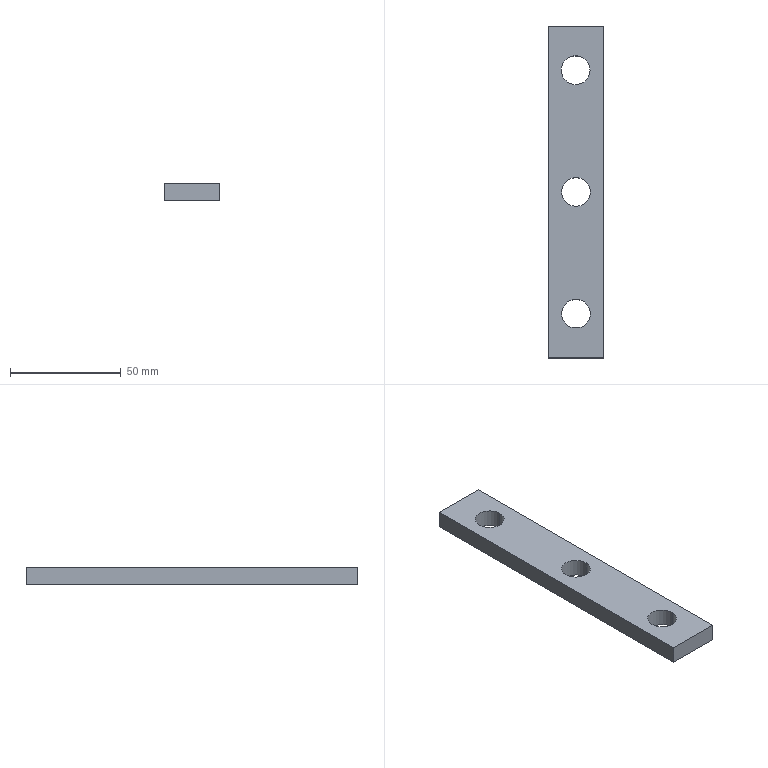Part | SolidWorks | features Extrusion 1 | 1 solid | 12 faces | box 25 x 150 x 8 mm | volume 26814 mm3 | cylinder 6 | plane 6 | commonest cylinder face diameters 13 x6
STEP:
#1=CARTESIAN_POINT('',(-6.5,-55.,8.));
#2=VERTEX_POINT('',#1);
#3=CARTESIAN_POINT('',(6.5,-55.,8.));
#4=VERTEX_POINT('',#3);
#5=CARTESIAN_POINT('',(0.,-55.,8.));
#6=DIRECTION('',(0.,0.,1.));
#7=DIRECTION('',(1.,0.,0.));
#8=AXIS2_PLACEMENT_3D('',#5,#6,#7);
#9=CIRCLE('',#8,6.5);
#10=EDGE_CURVE('',#2,#4,#9,.T.);
#11=ORIENTED_EDGE('',*,*,#10,.T.);
#12=CARTESIAN_POINT('',(6.5,-55.,0.));
#13=VERTEX_POINT('',#12);
#14=CARTESIAN_POINT('',(6.5,-55.,8.));
#15=DIRECTION('',(0.,0.,-1.));
#16=VECTOR('',#15,1000.);
#17=LINE('',#14,#16);
#18=EDGE_CURVE('',#4,#13,#17,.T.);
#19=ORIENTED_EDGE('',*,*,#18,.T.);
#20=CARTESIAN_POINT('',(-6.5,-55.,0.));
#21=VERTEX_POINT('',#20);
#22=CARTESIAN_POINT('',(0.,-55.,0.));
#23=DIRECTION('',(0.,0.,1.));
#24=DIRECTION('',(1.,0.,0.));
#25=AXIS2_PLACEMENT_3D('',#22,#23,#24);
#26=CIRCLE('',#25,6.5);
#27=EDGE_CURVE('',#21,#13,#26,.T.);
#28=ORIENTED_EDGE('',*,*,#27,.F.);
#29=CARTESIAN_POINT('',(-6.5,-55.,8.));
#30=DIRECTION('',(0.,0.,-1.));
#31=VECTOR('',#30,1000.);
#32=LINE('',#29,#31);
#33=EDGE_CURVE('',#2,#21,#32,.T.);
#34=ORIENTED_EDGE('',*,*,#33,.F.);
#35=EDGE_LOOP('',(#11,#19,#28,#34));
#36=FACE_OUTER_BOUND('',#35,.T.);
#37=CARTESIAN_POINT('',(0.,-55.,8.));
#38=DIRECTION('',(0.,0.,-1.));
#39=DIRECTION('',(-1.,0.,0.));
#40=AXIS2_PLACEMENT_3D('',#37,#38,#39);
#41=CYLINDRICAL_SURFACE('',#40,6.5);
#42=ADVANCED_FACE('',(#36),#41,.F.);
#43=CARTESIAN_POINT('',(-6.5,0.,8.));
#44=VERTEX_POINT('',#43);
#45=CARTESIAN_POINT('',(6.5,0.,8.));
#46=VERTEX_POINT('',#45);
#47=CARTESIAN_POINT('',(0.,0.,8.));
#48=DIRECTION('',(0.,0.,1.));
#49=DIRECTION('',(1.,0.,0.));
#50=AXIS2_PLACEMENT_3D('',#47,#48,#49);
#51=CIRCLE('',#50,6.5);
#52=EDGE_CURVE('',#44,#46,#51,.T.);
#53=ORIENTED_EDGE('',*,*,#52,.T.);
#54=CARTESIAN_POINT('',(6.5,0.,0.));
#55=VERTEX_POINT('',#54);
#56=CARTESIAN_POINT('',(6.5,0.,8.));
#57=DIRECTION('',(0.,0.,-1.));
#58=VECTOR('',#57,1000.);
#59=LINE('',#56,#58);
#60=EDGE_CURVE('',#46,#55,#59,.T.);
#61=ORIENTED_EDGE('',*,*,#60,.T.);
#62=CARTESIAN_POINT('',(-6.5,0.,0.));
#63=VERTEX_POINT('',#62);
#64=CARTESIAN_POINT('',(0.,0.,0.));
#65=DIRECTION('',(0.,0.,1.));
#66=DIRECTION('',(1.,0.,0.));
#67=AXIS2_PLACEMENT_3D('',#64,#65,#66);
#68=CIRCLE('',#67,6.5);
#69=EDGE_CURVE('',#63,#55,#68,.T.);
#70=ORIENTED_EDGE('',*,*,#69,.F.);
#71=CARTESIAN_POINT('',(-6.5,0.,8.));
#72=DIRECTION('',(0.,0.,-1.));
#73=VECTOR('',#72,1000.);
#74=LINE('',#71,#73);
#75=EDGE_CURVE('',#44,#63,#74,.T.);
#76=ORIENTED_EDGE('',*,*,#75,.F.);
#77=EDGE_LOOP('',(#53,#61,#70,#76));
#78=FACE_OUTER_BOUND('',#77,.T.);
#79=CARTESIAN_POINT('',(0.,0.,8.));
#80=DIRECTION('',(0.,0.,-1.));
#81=DIRECTION('',(-1.,0.,0.));
#82=AXIS2_PLACEMENT_3D('',#79,#80,#81);
#83=CYLINDRICAL_SURFACE('',#82,6.5);
#84=ADVANCED_FACE('',(#78),#83,.F.);
#85=CARTESIAN_POINT('',(-6.654,55.,8.));
#86=VERTEX_POINT('',#85);
#87=CARTESIAN_POINT('',(6.346,55.,8.));
#88=VERTEX_POINT('',#87);
#89=CARTESIAN_POINT('',(-0.1539,55.,8.));
#90=DIRECTION('',(0.,0.,1.));
#91=DIRECTION('',(1.,0.,0.));
#92=AXIS2_PLACEMENT_3D('',#89,#90,#91);
#93=CIRCLE('',#92,6.5);
#94=EDGE_CURVE('',#86,#88,#93,.T.);
#95=ORIENTED_EDGE('',*,*,#94,.T.);
#96=CARTESIAN_POINT('',(6.346,55.,0.));
#97=VERTEX_POINT('',#96);
#98=CARTESIAN_POINT('',(6.346,55.,8.));
#99=DIRECTION('',(0.,0.,-1.));
#100=VECTOR('',#99,1000.);
#101=LINE('',#98,#100);
#102=EDGE_CURVE('',#88,#97,#101,.T.);
#103=ORIENTED_EDGE('',*,*,#102,.T.);
#104=CARTESIAN_POINT('',(-6.654,55.,0.));
#105=VERTEX_POINT('',#104);
#106=CARTESIAN_POINT('',(-0.1539,55.,0.));
#107=DIRECTION('',(0.,0.,1.));
#108=DIRECTION('',(1.,0.,0.));
#109=AXIS2_PLACEMENT_3D('',#106,#107,#108);
#110=CIRCLE('',#109,6.5);
#111=EDGE_CURVE('',#105,#97,#110,.T.);
#112=ORIENTED_EDGE('',*,*,#111,.F.);
#113=CARTESIAN_POINT('',(-6.654,55.,8.));
#114=DIRECTION('',(0.,0.,-1.));
#115=VECTOR('',#114,1000.);
#116=LINE('',#113,#115);
#117=EDGE_CURVE('',#86,#105,#116,.T.);
#118=ORIENTED_EDGE('',*,*,#117,.F.);
#119=EDGE_LOOP('',(#95,#103,#112,#118));
#120=FACE_OUTER_BOUND('',#119,.T.);
#121=CARTESIAN_POINT('',(-0.1539,55.,8.));
#122=DIRECTION('',(0.,0.,-1.));
#123=DIRECTION('',(-1.,0.,0.));
#124=AXIS2_PLACEMENT_3D('',#121,#122,#123);
#125=CYLINDRICAL_SURFACE('',#124,6.5);
#126=ADVANCED_FACE('',(#120),#125,.F.);
#127=CARTESIAN_POINT('',(-12.5,75.,8.));
#128=VERTEX_POINT('',#127);
#129=CARTESIAN_POINT('',(-12.5,-75.,8.));
#130=VERTEX_POINT('',#129);
#131=CARTESIAN_POINT('',(-12.5,75.,8.));
#132=DIRECTION('',(0.,-1.,0.));
#133=VECTOR('',#132,1000.);
#134=LINE('',#131,#133);
#135=EDGE_CURVE('',#128,#130,#134,.T.);
#136=ORIENTED_EDGE('',*,*,#135,.T.);
#137=CARTESIAN_POINT('',(12.5,-75.,8.));
#138=VERTEX_POINT('',#137);
#139=CARTESIAN_POINT('',(12.5,-75.,8.));
#140=DIRECTION('',(1.,0.,0.));
#141=VECTOR('',#140,1000.);
#142=LINE('',#139,#141);
#143=EDGE_CURVE('',#130,#138,#142,.T.);
#144=ORIENTED_EDGE('',*,*,#143,.T.);
#145=CARTESIAN_POINT('',(12.5,75.,8.));
#146=VERTEX_POINT('',#145);
#147=CARTESIAN_POINT('',(12.5,75.,8.));
#148=DIRECTION('',(0.,1.,0.));
#149=VECTOR('',#148,1000.);
#150=LINE('',#147,#149);
#151=EDGE_CURVE('',#138,#146,#150,.T.);
#152=ORIENTED_EDGE('',*,*,#151,.T.);
#153=CARTESIAN_POINT('',(12.5,75.,8.));
#154=DIRECTION('',(-1.,0.,0.));
#155=VECTOR('',#154,1000.);
#156=LINE('',#153,#155);
#157=EDGE_CURVE('',#146,#128,#156,.T.);
#158=ORIENTED_EDGE('',*,*,#157,.T.);
#159=EDGE_LOOP('',(#136,#144,#152,#158));
#160=FACE_OUTER_BOUND('',#159,.T.);
#161=ORIENTED_EDGE('',*,*,#94,.F.);
#162=CARTESIAN_POINT('',(-0.1539,55.,8.));
#163=DIRECTION('',(0.,0.,1.));
#164=DIRECTION('',(1.,0.,0.));
#165=AXIS2_PLACEMENT_3D('',#162,#163,#164);
#166=CIRCLE('',#165,6.5);
#167=EDGE_CURVE('',#88,#86,#166,.T.);
#168=ORIENTED_EDGE('',*,*,#167,.F.);
#169=EDGE_LOOP('',(#161,#168));
#170=FACE_BOUND('',#169,.T.);
#171=ORIENTED_EDGE('',*,*,#52,.F.);
#172=CARTESIAN_POINT('',(0.,0.,8.));
#173=DIRECTION('',(0.,0.,1.));
#174=DIRECTION('',(1.,0.,0.));
#175=AXIS2_PLACEMENT_3D('',#172,#173,#174);
#176=CIRCLE('',#175,6.5);
#177=EDGE_CURVE('',#46,#44,#176,.T.);
#178=ORIENTED_EDGE('',*,*,#177,.F.);
#179=EDGE_LOOP('',(#171,#178));
#180=FACE_BOUND('',#179,.T.);
#181=ORIENTED_EDGE('',*,*,#10,.F.);
#182=CARTESIAN_POINT('',(0.,-55.,8.));
#183=DIRECTION('',(0.,0.,1.));
#184=DIRECTION('',(1.,0.,0.));
#185=AXIS2_PLACEMENT_3D('',#182,#183,#184);
#186=CIRCLE('',#185,6.5);
#187=EDGE_CURVE('',#4,#2,#186,.T.);
#188=ORIENTED_EDGE('',*,*,#187,.F.);
#189=EDGE_LOOP('',(#181,#188));
#190=FACE_BOUND('',#189,.T.);
#191=CARTESIAN_POINT('',(0.,0.,8.));
#192=DIRECTION('',(0.,0.,-1.));
#193=DIRECTION('',(-1.,0.,0.));
#194=AXIS2_PLACEMENT_3D('',#191,#192,#193);
#195=PLANE('',#194);
#196=ADVANCED_FACE('',(#160,#170,#180,#190),#195,.F.);
#197=ORIENTED_EDGE('',*,*,#69,.T.);
#198=CARTESIAN_POINT('',(0.,0.,0.));
#199=DIRECTION('',(0.,0.,1.));
#200=DIRECTION('',(1.,0.,0.));
#201=AXIS2_PLACEMENT_3D('',#198,#199,#200);
#202=CIRCLE('',#201,6.5);
#203=EDGE_CURVE('',#55,#63,#202,.T.);
#204=ORIENTED_EDGE('',*,*,#203,.T.);
#205=EDGE_LOOP('',(#197,#204));
#206=FACE_BOUND('',#205,.T.);
#207=CARTESIAN_POINT('',(-12.5,75.,0.));
#208=VERTEX_POINT('',#207);
#209=CARTESIAN_POINT('',(-12.5,-75.,0.));
#210=VERTEX_POINT('',#209);
#211=CARTESIAN_POINT('',(-12.5,75.,0.));
#212=DIRECTION('',(0.,-1.,0.));
#213=VECTOR('',#212,1000.);
#214=LINE('',#211,#213);
#215=EDGE_CURVE('',#208,#210,#214,.T.);
#216=ORIENTED_EDGE('',*,*,#215,.F.);
#217=CARTESIAN_POINT('',(12.5,75.,0.));
#218=VERTEX_POINT('',#217);
#219=CARTESIAN_POINT('',(12.5,75.,0.));
#220=DIRECTION('',(-1.,0.,0.));
#221=VECTOR('',#220,1000.);
#222=LINE('',#219,#221);
#223=EDGE_CURVE('',#218,#208,#222,.T.);
#224=ORIENTED_EDGE('',*,*,#223,.F.);
#225=CARTESIAN_POINT('',(12.5,-75.,0.));
#226=VERTEX_POINT('',#225);
#227=CARTESIAN_POINT('',(12.5,75.,0.));
#228=DIRECTION('',(0.,1.,0.));
#229=VECTOR('',#228,1000.);
#230=LINE('',#227,#229);
#231=EDGE_CURVE('',#226,#218,#230,.T.);
#232=ORIENTED_EDGE('',*,*,#231,.F.);
#233=CARTESIAN_POINT('',(12.5,-75.,0.));
#234=DIRECTION('',(1.,0.,0.));
#235=VECTOR('',#234,1000.);
#236=LINE('',#233,#235);
#237=EDGE_CURVE('',#210,#226,#236,.T.);
#238=ORIENTED_EDGE('',*,*,#237,.F.);
#239=EDGE_LOOP('',(#216,#224,#232,#238));
#240=FACE_OUTER_BOUND('',#239,.T.);
#241=ORIENTED_EDGE('',*,*,#111,.T.);
#242=CARTESIAN_POINT('',(-0.1539,55.,0.));
#243=DIRECTION('',(0.,0.,1.));
#244=DIRECTION('',(1.,0.,0.));
#245=AXIS2_PLACEMENT_3D('',#242,#243,#244);
#246=CIRCLE('',#245,6.5);
#247=EDGE_CURVE('',#97,#105,#246,.T.);
#248=ORIENTED_EDGE('',*,*,#247,.T.);
#249=EDGE_LOOP('',(#241,#248));
#250=FACE_BOUND('',#249,.T.);
#251=ORIENTED_EDGE('',*,*,#27,.T.);
#252=CARTESIAN_POINT('',(0.,-55.,0.));
#253=DIRECTION('',(0.,0.,1.));
#254=DIRECTION('',(1.,0.,0.));
#255=AXIS2_PLACEMENT_3D('',#252,#253,#254);
#256=CIRCLE('',#255,6.5);
#257=EDGE_CURVE('',#13,#21,#256,.T.);
#258=ORIENTED_EDGE('',*,*,#257,.T.);
#259=EDGE_LOOP('',(#251,#258));
#260=FACE_BOUND('',#259,.T.);
#261=CARTESIAN_POINT('',(0.,0.,0.));
#262=DIRECTION('',(0.,0.,-1.));
#263=DIRECTION('',(-1.,0.,0.));
#264=AXIS2_PLACEMENT_3D('',#261,#262,#263);
#265=PLANE('',#264);
#266=ADVANCED_FACE('',(#206,#240,#250,#260),#265,.T.);
#267=ORIENTED_EDGE('',*,*,#215,.T.);
#268=CARTESIAN_POINT('',(-12.5,-75.,8.));
#269=DIRECTION('',(0.,0.,-1.));
#270=VECTOR('',#269,1000.);
#271=LINE('',#268,#270);
#272=EDGE_CURVE('',#130,#210,#271,.T.);
#273=ORIENTED_EDGE('',*,*,#272,.F.);
#274=ORIENTED_EDGE('',*,*,#135,.F.);
#275=CARTESIAN_POINT('',(-12.5,75.,8.));
#276=DIRECTION('',(0.,0.,-1.));
#277=VECTOR('',#276,1000.);
#278=LINE('',#275,#277);
#279=EDGE_CURVE('',#128,#208,#278,.T.);
#280=ORIENTED_EDGE('',*,*,#279,.T.);
#281=EDGE_LOOP('',(#267,#273,#274,#280));
#282=FACE_OUTER_BOUND('',#281,.T.);
#283=CARTESIAN_POINT('',(-12.5,75.,8.));
#284=DIRECTION('',(1.,0.,0.));
#285=DIRECTION('',(0.,1.,0.));
#286=AXIS2_PLACEMENT_3D('',#283,#284,#285);
#287=PLANE('',#286);
#288=ADVANCED_FACE('',(#282),#287,.F.);
#289=ORIENTED_EDGE('',*,*,#237,.T.);
#290=CARTESIAN_POINT('',(12.5,-75.,8.));
#291=DIRECTION('',(0.,0.,-1.));
#292=VECTOR('',#291,1000.);
#293=LINE('',#290,#292);
#294=EDGE_CURVE('',#138,#226,#293,.T.);
#295=ORIENTED_EDGE('',*,*,#294,.F.);
#296=ORIENTED_EDGE('',*,*,#143,.F.);
#297=ORIENTED_EDGE('',*,*,#272,.T.);
#298=EDGE_LOOP('',(#289,#295,#296,#297));
#299=FACE_OUTER_BOUND('',#298,.T.);
#300=CARTESIAN_POINT('',(12.5,-75.,8.));
#301=DIRECTION('',(0.,1.,0.));
#302=DIRECTION('',(0.,0.,1.));
#303=AXIS2_PLACEMENT_3D('',#300,#301,#302);
#304=PLANE('',#303);
#305=ADVANCED_FACE('',(#299),#304,.F.);
#306=ORIENTED_EDGE('',*,*,#231,.T.);
#307=CARTESIAN_POINT('',(12.5,75.,8.));
#308=DIRECTION('',(0.,0.,-1.));
#309=VECTOR('',#308,1000.);
#310=LINE('',#307,#309);
#311=EDGE_CURVE('',#146,#218,#310,.T.);
#312=ORIENTED_EDGE('',*,*,#311,.F.);
#313=ORIENTED_EDGE('',*,*,#151,.F.);
#314=ORIENTED_EDGE('',*,*,#294,.T.);
#315=EDGE_LOOP('',(#306,#312,#313,#314));
#316=FACE_OUTER_BOUND('',#315,.T.);
#317=CARTESIAN_POINT('',(12.5,75.,8.));
#318=DIRECTION('',(-1.,0.,0.));
#319=DIRECTION('',(0.,-1.,0.));
#320=AXIS2_PLACEMENT_3D('',#317,#318,#319);
#321=PLANE('',#320);
#322=ADVANCED_FACE('',(#316),#321,.F.);
#323=ORIENTED_EDGE('',*,*,#223,.T.);
#324=ORIENTED_EDGE('',*,*,#279,.F.);
#325=ORIENTED_EDGE('',*,*,#157,.F.);
#326=ORIENTED_EDGE('',*,*,#311,.T.);
#327=EDGE_LOOP('',(#323,#324,#325,#326));
#328=FACE_OUTER_BOUND('',#327,.T.);
#329=CARTESIAN_POINT('',(12.5,75.,8.));
#330=DIRECTION('',(0.,-1.,0.));
#331=DIRECTION('',(0.,0.,-1.));
#332=AXIS2_PLACEMENT_3D('',#329,#330,#331);
#333=PLANE('',#332);
#334=ADVANCED_FACE('',(#328),#333,.F.);
#335=ORIENTED_EDGE('',*,*,#102,.F.);
#336=ORIENTED_EDGE('',*,*,#167,.T.);
#337=ORIENTED_EDGE('',*,*,#117,.T.);
#338=ORIENTED_EDGE('',*,*,#247,.F.);
#339=EDGE_LOOP('',(#335,#336,#337,#338));
#340=FACE_OUTER_BOUND('',#339,.T.);
#341=CARTESIAN_POINT('',(-0.1539,55.,8.));
#342=DIRECTION('',(0.,0.,-1.));
#343=DIRECTION('',(-1.,0.,0.));
#344=AXIS2_PLACEMENT_3D('',#341,#342,#343);
#345=CYLINDRICAL_SURFACE('',#344,6.5);
#346=ADVANCED_FACE('',(#340),#345,.F.);
#347=ORIENTED_EDGE('',*,*,#60,.F.);
#348=ORIENTED_EDGE('',*,*,#177,.T.);
#349=ORIENTED_EDGE('',*,*,#75,.T.);
#350=ORIENTED_EDGE('',*,*,#203,.F.);
#351=EDGE_LOOP('',(#347,#348,#349,#350));
#352=FACE_OUTER_BOUND('',#351,.T.);
#353=CARTESIAN_POINT('',(0.,0.,8.));
#354=DIRECTION('',(0.,0.,-1.));
#355=DIRECTION('',(-1.,0.,0.));
#356=AXIS2_PLACEMENT_3D('',#353,#354,#355);
#357=CYLINDRICAL_SURFACE('',#356,6.5);
#358=ADVANCED_FACE('',(#352),#357,.F.);
#359=ORIENTED_EDGE('',*,*,#18,.F.);
#360=ORIENTED_EDGE('',*,*,#187,.T.);
#361=ORIENTED_EDGE('',*,*,#33,.T.);
#362=ORIENTED_EDGE('',*,*,#257,.F.);
#363=EDGE_LOOP('',(#359,#360,#361,#362));
#364=FACE_OUTER_BOUND('',#363,.T.);
#365=CARTESIAN_POINT('',(0.,-55.,8.));
#366=DIRECTION('',(0.,0.,-1.));
#367=DIRECTION('',(-1.,0.,0.));
#368=AXIS2_PLACEMENT_3D('',#365,#366,#367);
#369=CYLINDRICAL_SURFACE('',#368,6.5);
#370=ADVANCED_FACE('',(#364),#369,.F.);
#371=CLOSED_SHELL('',(#42,#84,#126,#196,#266,#288,#305,#322,#334,#346,#358,#370));
#372=MANIFOLD_SOLID_BREP('',#371);
#373=CARTESIAN_POINT('',(0.,0.,0.));
#374=DIRECTION('',(0.,0.,1.));
#375=DIRECTION('',(1.,0.,0.));
#376=AXIS2_PLACEMENT_3D('',#373,#374,#375);
#377=(LENGTH_UNIT()NAMED_UNIT(*)SI_UNIT(.MILLI.,.METRE.));
#378=UNCERTAINTY_MEASURE_WITH_UNIT(LENGTH_MEASURE(0.00001),#377,'','');
#379=(NAMED_UNIT(*)PLANE_ANGLE_UNIT()SI_UNIT($,.RADIAN.));
#380=(NAMED_UNIT(*)SI_UNIT($,.STERADIAN.)SOLID_ANGLE_UNIT());
#381=(GEOMETRIC_REPRESENTATION_CONTEXT(3)GLOBAL_UNCERTAINTY_ASSIGNED_CONTEXT((#378))GLOBAL_UNIT_ASSIGNED_CONTEXT((#377,#379,#380))REPRESENTATION_CONTEXT('',''));
#382=ADVANCED_BREP_SHAPE_REPRESENTATION('',(#372,#376),#381);